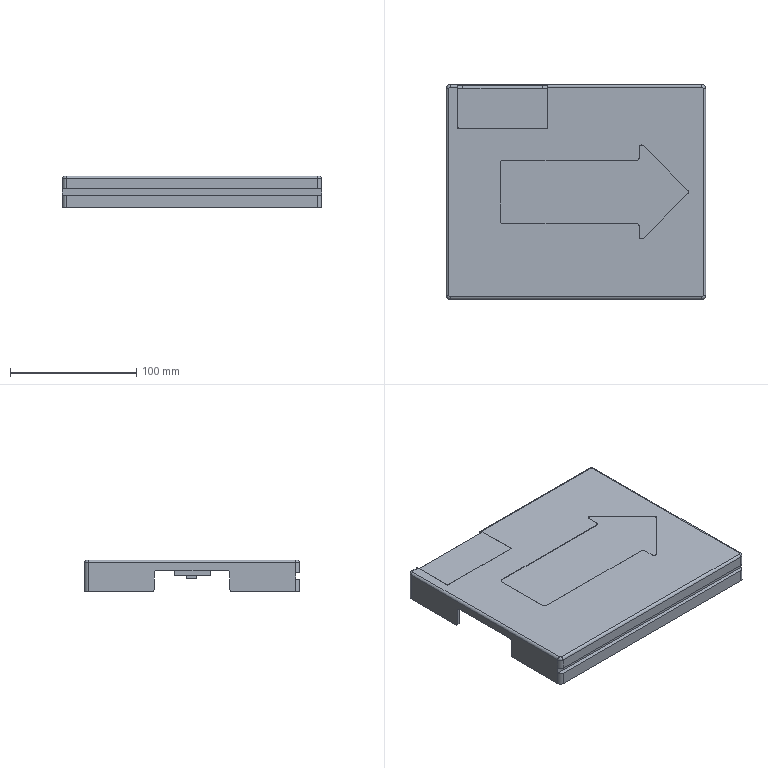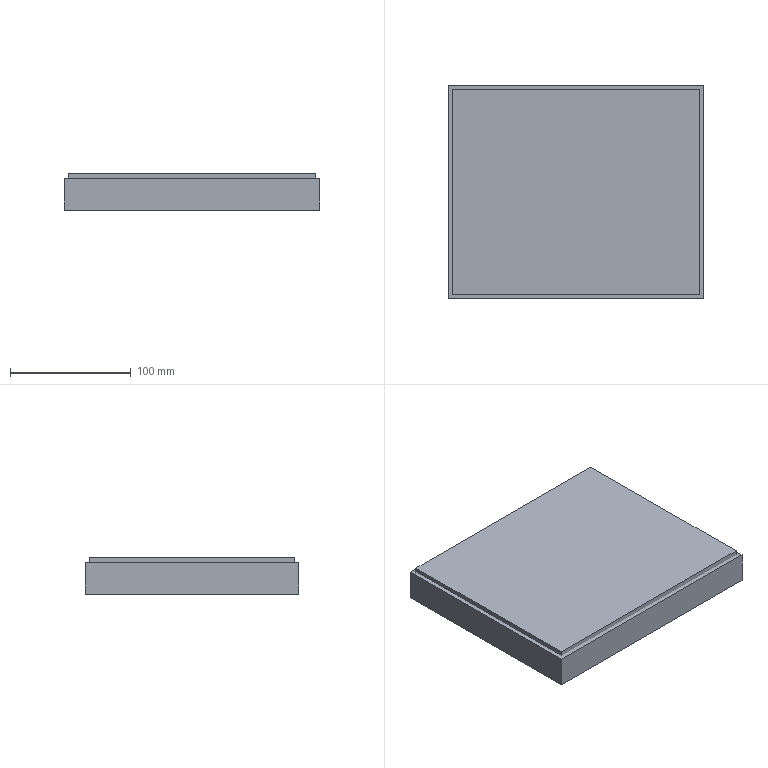CAM job | NX | 3+2 milling, drilling | part box 205 x 170 x 25 mm | stock box 212 x 177 x 30 mm
Tools:
number,name,description,diameter,corner_radius,flute_length,length,flutes
3,D63,Milling Tool-5 Parameters,63.0,0.0,50.0,75.0,2
4,D10,Milling Tool-5 Parameters,10.0,0.0,50.0,75.0,2
17,D4,Milling Tool-5 Parameters,4.0,0.0,50.0,75.0,2
14,D10JING,Milling Tool-5 Parameters,10.0,0.0,50.0,75.0,2
7,D3R0.5,Milling Tool-5 Parameters,3.0,0.5,50.0,75.0,2
1,D6A45,Milling Tool-5 Parameters,6.0,0.0,3.0,3.0,2
13,T10H1.5,Milling Tool-T Cutter,10.0,,1.5,20.0,4
22,2.5ZT,Drilling Tool,2.5,0.0,35.0,50.0,2
Operations:
program,operation,operation_type,tool,method,geometry_group,spindle_rpm,surface_speed,feed_per_tooth,feed_cut,feed_plunge,cut_length_mm,path_length_mm,cut_time_min,machine_time_min
1_1,FLOOR_WALL,VolumeBased25DMillingOperation,D63,METHOD,A,6500.0,1286.0,0.0962,1250.0,100.0,1538.797,1592.797,1.231,1.236
1_1,ADAPTIVE_MILLING,CavityMilling,D10,METHOD,A,9500.0,298.0,0.1579,3000.0,1000.0,6283.661,6474.298,2.096,2.115
1_1,FLOOR_WALL_1,VolumeBased25DMillingOperation,D10,METHOD,A,9500.0,298.0,0.1316,2500.0,1000.0,1150.594,1205.494,0.5107,0.5162
1_1,FLOOR_WALL_1_COPY,VolumeBased25DMillingOperation,D10,METHOD,A,9500.0,298.0,0.1316,2500.0,1000.0,449.558,507.458,0.2073,0.2131
1_1,CAVITY_MILL,CavityMilling,D4,METHOD,A,9500.0,119.0,0.0842,1600.0,100.0,288.839,1077.091,0.1805,0.2593
1_1,FLOOR_WALL_1_COPY_1,VolumeBased25DMillingOperation,D10JING,METHOD,A,9500.0,298.0,0.0632,1200.0,1000.0,1963.267,2181.954,1.639,1.661
1_1,ZLEVEL_PROFILE,ZLevelMilling,D10JING,METHOD,A,9500.0,298.0,0.0526,1000.0,100.0,1575.117,1679.553,1.575,1.586
1_1,ZLEVEL_PROFILE_1,ZLevelMilling,D3R0.5,METHOD,A,9500.0,89.0,0.1316,2500.0,1000.0,28504.699,28624.038,11.404,11.416
1_1,ZLEVEL_PROFILE_1_COPY,ZLevelMilling,D3R0.5,METHOD,A,9500.0,89.0,0.1316,2500.0,1000.0,2592.729,2655.239,1.038,1.044
1_1,PLANAR_MILL_COPY_COPY,PlanarMilling,D6A45,METHOD,A,9500.0,179.0,0.0658,1250.0,100.0,141.179,200.779,0.1129,0.1189
1_1,PLANAR_MILL_COPY_COPY_COPY,PlanarMilling,D6A45,METHOD,A,9500.0,179.0,0.0658,1250.0,100.0,401.166,459.866,0.3209,0.3268
1_1,PLANAR_MILL_1,PlanarMilling,T10H1.5,METHOD,A,6500.0,204.0,0.0481,1250.0,100.0,9721.835,18995.736,7.777,8.705
2,DRILLING_COPY_1,Operation,D6A45,METHOD,B,5000.0,94.0,0.025,250.0,0.0,10.8,181.851,0.0432,0.0603
2,DRILLING_COPY_COPY,Operation,2.5ZT,METHOD,B,1447.0,10.0,0.0346,100.0,0.0,30.753,221.757,0.3075,0.3266
2,FLOOR_WALL_1_COPY_COPY,VolumeBased25DMillingOperation,D4,METHOD,B,9500.0,119.0,0.0763,1450.0,1000.0,2172.39,2264.66,1.531,1.54
2,ZLEVEL_PROFILE_COPY,ZLevelMilling,D4,METHOD,B,9500.0,298.0,0.0526,1000.0,100.0,2331.574,2405.608,2.332,2.339
3,FLOOR_WALL_COPY,VolumeBased25DMillingOperation,D63,METHOD,C,6500.0,1286.0,0.0962,1250.0,100.0,6143.985,6972.274,4.915,4.998
3,FLOOR_WALL_COPY_1,VolumeBased25DMillingOperation,D63,METHOD,C,6500.0,1286.0,0.0962,1250.0,100.0,1228.797,1282.797,0.983,0.9884
3,CAVITY_MILL_1,CavityMilling,D10,METHOD,C,9500.0,298.0,0.1579,3000.0,1000.0,124062.148,126032.277,41.691,41.888
3,CAVITY_MILL_1_COPY,CavityMilling,D4,METHOD,C,9500.0,119.0,0.0842,1600.0,1000.0,9021.577,13380.23,5.918,6.354
3,ZLEVEL_PROFILE_COPY_1,ZLevelMilling,D4,METHOD,C,9500.0,298.0,0.0526,1000.0,100.0,568.94,803.272,0.5689,0.5924
3,ZLEVEL_PROFILE_COPY_1_COPY,ZLevelMilling,D4,METHOD,C,9500.0,298.0,0.0526,1000.0,100.0,751.374,847.374,0.7514,0.761
3,ZLEVEL_PROFILE_COPY_1_COPY_1,ZLevelMilling,D4,METHOD,C,9500.0,298.0,0.0526,1000.0,100.0,185.81,287.81,0.1858,0.196
3,FLOOR_WALL_1_COPY_1_COPY,VolumeBased25DMillingOperation,D4,METHOD,C,9500.0,298.0,0.0632,1200.0,1000.0,14756.894,19383.515,12.34,12.818
3,ZLEVEL_PROFILE_1_COPY_1,ZLevelMilling,D3R0.5,METHOD,C,9500.0,89.0,0.1316,2500.0,1000.0,2428.057,3457.924,0.9793,1.082
3,DRILLING_COPY_1_COPY,Operation,D6A45,METHOD,C,5000.0,94.0,0.025,250.0,0.0,43.2,772.321,0.1728,0.2457
3,DRILLING_COPY_COPY_COPY,Operation,2.5ZT,METHOD,C,1447.0,10.0,0.0346,100.0,0.0,126.013,935.065,1.26,1.341
3,ZLEVEL_PROFILE_2,ZLevelMilling,D6A45,METHOD,C,9500.0,179.0,0.0658,1250.0,100.0,1183.49,2483.614,0.9468,1.077
3,ZLEVEL_PROFILE_2_COPY,ZLevelMilling,D6A45,METHOD,C,9500.0,179.0,0.0658,1250.0,100.0,133.057,508.907,0.1064,0.144
3,ZLEVEL_PROFILE_2_COPY_COPY,ZLevelMilling,D6A45,METHOD,C,9500.0,179.0,0.0658,1250.0,100.0,128.354,212.954,0.1027,0.1111
3,ZLEVEL_PROFILE_2_COPY_COPY_COPY,ZLevelMilling,D6A45,METHOD,C,9500.0,179.0,0.0658,1250.0,100.0,120.724,320.101,0.0966,0.1165